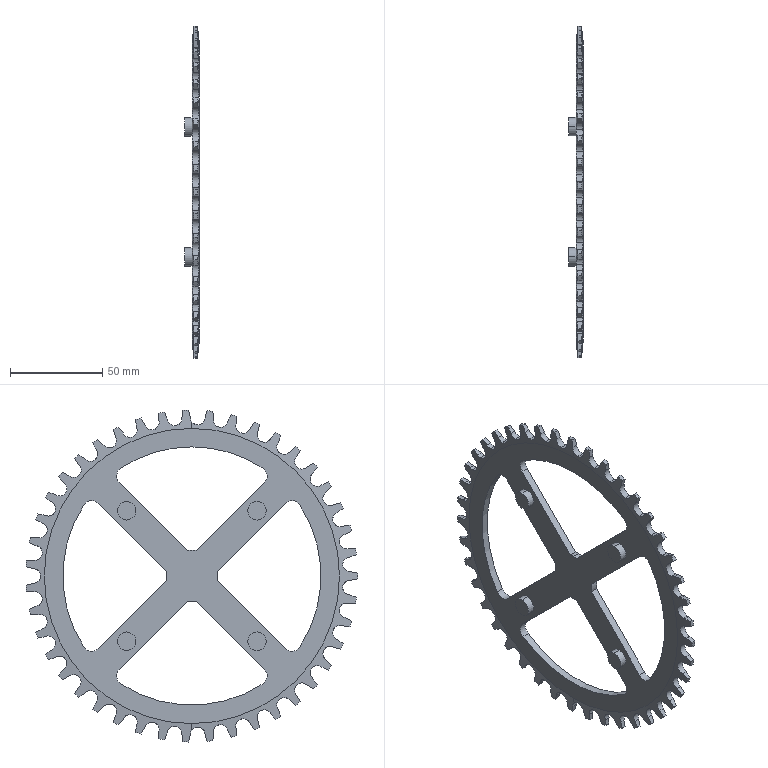Part | STEP file | Front gears | 1 solid | 239 faces | box 8 x 179.861 x 179.967 mm | volume 46199 mm3 | cylinder 135 | plane 100 | cone 4 | commonest cylinder face diameters 8 x64 180 x43 10 x18 28 x5 140 x5